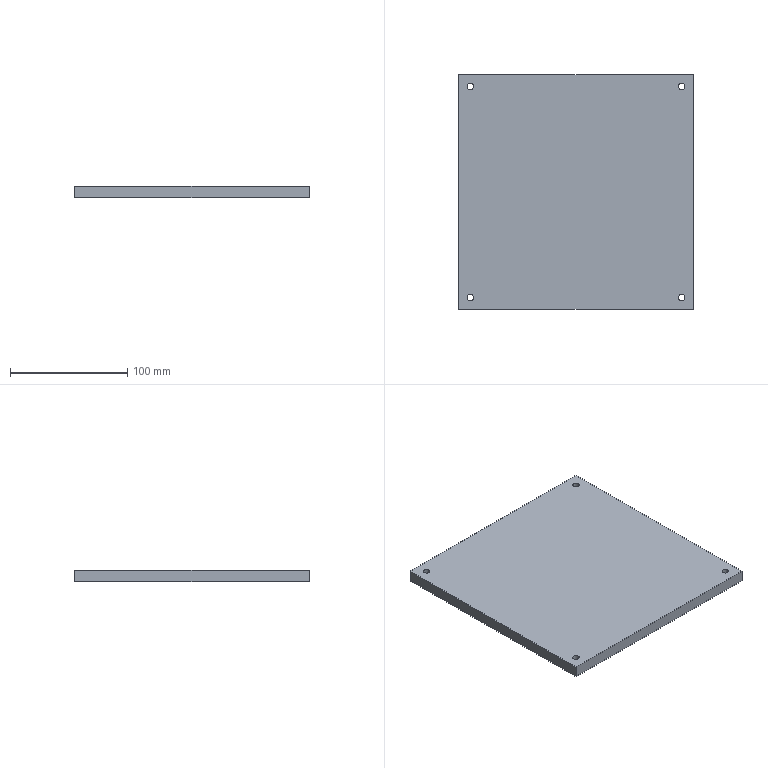Part | STEP file | B1-018 | 1 solid | 14 faces | box 200 x 200 x 10 mm | volume 399050 mm3 | cylinder 8 | plane 6 | commonest cylinder face diameters 5.5 x8
STEP:
#1=CARTESIAN_POINT('',(0.,0.,0.));
#2=DIRECTION('',(0.,0.,1.));
#3=DIRECTION('',(1.,0.,0.));
#4=AXIS2_PLACEMENT_3D('',#1,#2,#3);
#5=CARTESIAN_POINT('',(-87.25,90.,-5.));
#6=VERTEX_POINT('',#5);
#7=CARTESIAN_POINT('',(-87.25,90.,5.));
#8=VERTEX_POINT('',#7);
#9=CARTESIAN_POINT('',(-87.25,90.,-12.778));
#10=DIRECTION('',(0.,0.,1.));
#11=VECTOR('',#10,1.);
#12=LINE('',#9,#11);
#13=CARTESIAN_POINT('',(-90.,90.,-12.778));
#14=DIRECTION('',(0.,0.,1.));
#15=DIRECTION('',(1.,0.,0.));
#16=AXIS2_PLACEMENT_3D('',#13,#14,#15);
#17=CYLINDRICAL_SURFACE('',#16,2.75);
#18=CARTESIAN_POINT('',(6.283,0.));
#19=DIRECTION('',(0.,1.));
#20=VECTOR('',#19,1.);
#21=LINE('',#18,#20);
#22=(GEOMETRIC_REPRESENTATION_CONTEXT(2)PARAMETRIC_REPRESENTATION_CONTEXT()REPRESENTATION_CONTEXT('',''));
#23=DEFINITIONAL_REPRESENTATION('',(#21),#22);
#24=PCURVE('',#17,#23);
#25=CARTESIAN_POINT('',(-90.,90.,-12.778));
#26=DIRECTION('',(0.,0.,1.));
#27=DIRECTION('',(1.,0.,0.));
#28=AXIS2_PLACEMENT_3D('',#25,#26,#27);
#29=CYLINDRICAL_SURFACE('',#28,2.75);
#30=CARTESIAN_POINT('',(0.,0.));
#31=DIRECTION('',(0.,1.));
#32=VECTOR('',#31,1.);
#33=LINE('',#30,#32);
#34=(GEOMETRIC_REPRESENTATION_CONTEXT(2)PARAMETRIC_REPRESENTATION_CONTEXT()REPRESENTATION_CONTEXT('',''));
#35=DEFINITIONAL_REPRESENTATION('',(#33),#34);
#36=PCURVE('',#29,#35);
#37=SURFACE_CURVE('',#12,(#24,#36),.PCURVE_S1.);
#38=EDGE_CURVE('',#6,#8,#37,.T.);
#39=ORIENTED_EDGE('',*,*,#38,.T.);
#40=CARTESIAN_POINT('',(-92.75,90.,5.));
#41=VERTEX_POINT('',#40);
#42=CARTESIAN_POINT('',(-90.,90.,5.));
#43=DIRECTION('',(0.,0.,1.));
#44=DIRECTION('',(1.,0.,0.));
#45=AXIS2_PLACEMENT_3D('',#42,#43,#44);
#46=CIRCLE('',#45,2.75);
#47=CARTESIAN_POINT('',(0.,17.778));
#48=DIRECTION('',(1.,0.));
#49=VECTOR('',#48,1.);
#50=LINE('',#47,#49);
#51=(GEOMETRIC_REPRESENTATION_CONTEXT(2)PARAMETRIC_REPRESENTATION_CONTEXT()REPRESENTATION_CONTEXT('',''));
#52=DEFINITIONAL_REPRESENTATION('',(#50),#51);
#53=PCURVE('',#17,#52);
#54=CARTESIAN_POINT('',(0.,0.,5.));
#55=DIRECTION('',(0.,0.,1.));
#56=DIRECTION('',(1.,0.,0.));
#57=AXIS2_PLACEMENT_3D('',#54,#55,#56);
#58=PLANE('',#57);
#59=CARTESIAN_POINT('',(-90.,90.));
#60=DIRECTION('',(1.,0.));
#61=AXIS2_PLACEMENT_2D('',#59,#60);
#62=CIRCLE('',#61,2.75);
#63=(GEOMETRIC_REPRESENTATION_CONTEXT(2)PARAMETRIC_REPRESENTATION_CONTEXT()REPRESENTATION_CONTEXT('',''));
#64=DEFINITIONAL_REPRESENTATION('',(#62),#63);
#65=PCURVE('',#58,#64);
#66=SURFACE_CURVE('',#46,(#53,#65),.PCURVE_S1.);
#67=EDGE_CURVE('',#41,#8,#66,.T.);
#68=ORIENTED_EDGE('',*,*,#67,.F.);
#69=CARTESIAN_POINT('',(-92.75,90.,-5.));
#70=VERTEX_POINT('',#69);
#71=CARTESIAN_POINT('',(-92.75,90.,-12.778));
#72=DIRECTION('',(0.,0.,1.));
#73=VECTOR('',#72,1.);
#74=LINE('',#71,#73);
#75=CARTESIAN_POINT('',(3.142,0.));
#76=DIRECTION('',(0.,1.));
#77=VECTOR('',#76,1.);
#78=LINE('',#75,#77);
#79=(GEOMETRIC_REPRESENTATION_CONTEXT(2)PARAMETRIC_REPRESENTATION_CONTEXT()REPRESENTATION_CONTEXT('',''));
#80=DEFINITIONAL_REPRESENTATION('',(#78),#79);
#81=PCURVE('',#17,#80);
#82=CARTESIAN_POINT('',(3.142,0.));
#83=DIRECTION('',(0.,1.));
#84=VECTOR('',#83,1.);
#85=LINE('',#82,#84);
#86=(GEOMETRIC_REPRESENTATION_CONTEXT(2)PARAMETRIC_REPRESENTATION_CONTEXT()REPRESENTATION_CONTEXT('',''));
#87=DEFINITIONAL_REPRESENTATION('',(#85),#86);
#88=PCURVE('',#29,#87);
#89=SURFACE_CURVE('',#74,(#81,#88),.PCURVE_S1.);
#90=EDGE_CURVE('',#70,#41,#89,.T.);
#91=ORIENTED_EDGE('',*,*,#90,.F.);
#92=CARTESIAN_POINT('',(-90.,90.,-5.));
#93=DIRECTION('',(0.,0.,-1.));
#94=DIRECTION('',(1.,0.,0.));
#95=AXIS2_PLACEMENT_3D('',#92,#93,#94);
#96=CIRCLE('',#95,2.75);
#97=CARTESIAN_POINT('',(6.283,7.778));
#98=DIRECTION('',(-1.,0.));
#99=VECTOR('',#98,1.);
#100=LINE('',#97,#99);
#101=(GEOMETRIC_REPRESENTATION_CONTEXT(2)PARAMETRIC_REPRESENTATION_CONTEXT()REPRESENTATION_CONTEXT('',''));
#102=DEFINITIONAL_REPRESENTATION('',(#100),#101);
#103=PCURVE('',#17,#102);
#104=CARTESIAN_POINT('',(0.,0.,-5.));
#105=DIRECTION('',(0.,0.,1.));
#106=DIRECTION('',(1.,0.,0.));
#107=AXIS2_PLACEMENT_3D('',#104,#105,#106);
#108=PLANE('',#107);
#109=CARTESIAN_POINT('',(-87.25,90.));
#110=CARTESIAN_POINT('',(-87.25,85.237));
#111=CARTESIAN_POINT('',(-91.375,87.618));
#112=CARTESIAN_POINT('',(-95.5,90.));
#113=CARTESIAN_POINT('',(-91.375,92.382));
#114=CARTESIAN_POINT('',(-87.25,94.763));
#115=CARTESIAN_POINT('',(-87.25,90.));
#116=(BOUNDED_CURVE()B_SPLINE_CURVE(2,(#109,#110,#111,#112,#113,#114,#115),.UNSPECIFIED.,.T.,.F.)B_SPLINE_CURVE_WITH_KNOTS((1,2,2,2,2,1),(-2.094,0.,2.094,4.189,6.283,8.378),.UNSPECIFIED.)CURVE()GEOMETRIC_REPRESENTATION_ITEM()RATIONAL_B_SPLINE_CURVE((1.,0.5,1.,0.5,1.,0.5,1.))REPRESENTATION_ITEM(''));
#117=(GEOMETRIC_REPRESENTATION_CONTEXT(2)PARAMETRIC_REPRESENTATION_CONTEXT()REPRESENTATION_CONTEXT('',''));
#118=DEFINITIONAL_REPRESENTATION('',(#116),#117);
#119=PCURVE('',#108,#118);
#120=SURFACE_CURVE('',#96,(#103,#119),.PCURVE_S1.);
#121=EDGE_CURVE('',#6,#70,#120,.T.);
#122=ORIENTED_EDGE('',*,*,#121,.F.);
#123=EDGE_LOOP('',(#39,#68,#91,#122));
#124=FACE_BOUND('',#123,.F.);
#125=ADVANCED_FACE('',(#124),#17,.F.);
#126=CARTESIAN_POINT('',(-87.25,-90.,-5.));
#127=VERTEX_POINT('',#126);
#128=CARTESIAN_POINT('',(-87.25,-90.,5.));
#129=VERTEX_POINT('',#128);
#130=CARTESIAN_POINT('',(-87.25,-90.,-12.778));
#131=DIRECTION('',(0.,0.,1.));
#132=VECTOR('',#131,1.);
#133=LINE('',#130,#132);
#134=CARTESIAN_POINT('',(-90.,-90.,-12.778));
#135=DIRECTION('',(0.,0.,1.));
#136=DIRECTION('',(1.,0.,0.));
#137=AXIS2_PLACEMENT_3D('',#134,#135,#136);
#138=CYLINDRICAL_SURFACE('',#137,2.75);
#139=CARTESIAN_POINT('',(6.283,0.));
#140=DIRECTION('',(0.,1.));
#141=VECTOR('',#140,1.);
#142=LINE('',#139,#141);
#143=(GEOMETRIC_REPRESENTATION_CONTEXT(2)PARAMETRIC_REPRESENTATION_CONTEXT()REPRESENTATION_CONTEXT('',''));
#144=DEFINITIONAL_REPRESENTATION('',(#142),#143);
#145=PCURVE('',#138,#144);
#146=CARTESIAN_POINT('',(-90.,-90.,-12.778));
#147=DIRECTION('',(0.,0.,1.));
#148=DIRECTION('',(1.,0.,0.));
#149=AXIS2_PLACEMENT_3D('',#146,#147,#148);
#150=CYLINDRICAL_SURFACE('',#149,2.75);
#151=CARTESIAN_POINT('',(0.,0.));
#152=DIRECTION('',(0.,1.));
#153=VECTOR('',#152,1.);
#154=LINE('',#151,#153);
#155=(GEOMETRIC_REPRESENTATION_CONTEXT(2)PARAMETRIC_REPRESENTATION_CONTEXT()REPRESENTATION_CONTEXT('',''));
#156=DEFINITIONAL_REPRESENTATION('',(#154),#155);
#157=PCURVE('',#150,#156);
#158=SURFACE_CURVE('',#133,(#145,#157),.PCURVE_S1.);
#159=EDGE_CURVE('',#127,#129,#158,.T.);
#160=ORIENTED_EDGE('',*,*,#159,.T.);
#161=CARTESIAN_POINT('',(-92.75,-90.,5.));
#162=VERTEX_POINT('',#161);
#163=CARTESIAN_POINT('',(-90.,-90.,5.));
#164=DIRECTION('',(0.,0.,1.));
#165=DIRECTION('',(1.,0.,0.));
#166=AXIS2_PLACEMENT_3D('',#163,#164,#165);
#167=CIRCLE('',#166,2.75);
#168=CARTESIAN_POINT('',(0.,17.778));
#169=DIRECTION('',(1.,0.));
#170=VECTOR('',#169,1.);
#171=LINE('',#168,#170);
#172=(GEOMETRIC_REPRESENTATION_CONTEXT(2)PARAMETRIC_REPRESENTATION_CONTEXT()REPRESENTATION_CONTEXT('',''));
#173=DEFINITIONAL_REPRESENTATION('',(#171),#172);
#174=PCURVE('',#138,#173);
#175=CARTESIAN_POINT('',(-90.,-90.));
#176=DIRECTION('',(1.,0.));
#177=AXIS2_PLACEMENT_2D('',#175,#176);
#178=CIRCLE('',#177,2.75);
#179=(GEOMETRIC_REPRESENTATION_CONTEXT(2)PARAMETRIC_REPRESENTATION_CONTEXT()REPRESENTATION_CONTEXT('',''));
#180=DEFINITIONAL_REPRESENTATION('',(#178),#179);
#181=PCURVE('',#58,#180);
#182=SURFACE_CURVE('',#167,(#174,#181),.PCURVE_S1.);
#183=EDGE_CURVE('',#162,#129,#182,.T.);
#184=ORIENTED_EDGE('',*,*,#183,.F.);
#185=CARTESIAN_POINT('',(-92.75,-90.,-5.));
#186=VERTEX_POINT('',#185);
#187=CARTESIAN_POINT('',(-92.75,-90.,-12.778));
#188=DIRECTION('',(0.,0.,1.));
#189=VECTOR('',#188,1.);
#190=LINE('',#187,#189);
#191=CARTESIAN_POINT('',(3.142,0.));
#192=DIRECTION('',(0.,1.));
#193=VECTOR('',#192,1.);
#194=LINE('',#191,#193);
#195=(GEOMETRIC_REPRESENTATION_CONTEXT(2)PARAMETRIC_REPRESENTATION_CONTEXT()REPRESENTATION_CONTEXT('',''));
#196=DEFINITIONAL_REPRESENTATION('',(#194),#195);
#197=PCURVE('',#138,#196);
#198=CARTESIAN_POINT('',(3.142,0.));
#199=DIRECTION('',(0.,1.));
#200=VECTOR('',#199,1.);
#201=LINE('',#198,#200);
#202=(GEOMETRIC_REPRESENTATION_CONTEXT(2)PARAMETRIC_REPRESENTATION_CONTEXT()REPRESENTATION_CONTEXT('',''));
#203=DEFINITIONAL_REPRESENTATION('',(#201),#202);
#204=PCURVE('',#150,#203);
#205=SURFACE_CURVE('',#190,(#197,#204),.PCURVE_S1.);
#206=EDGE_CURVE('',#186,#162,#205,.T.);
#207=ORIENTED_EDGE('',*,*,#206,.F.);
#208=CARTESIAN_POINT('',(-90.,-90.,-5.));
#209=DIRECTION('',(0.,0.,-1.));
#210=DIRECTION('',(1.,0.,0.));
#211=AXIS2_PLACEMENT_3D('',#208,#209,#210);
#212=CIRCLE('',#211,2.75);
#213=CARTESIAN_POINT('',(6.283,7.778));
#214=DIRECTION('',(-1.,0.));
#215=VECTOR('',#214,1.);
#216=LINE('',#213,#215);
#217=(GEOMETRIC_REPRESENTATION_CONTEXT(2)PARAMETRIC_REPRESENTATION_CONTEXT()REPRESENTATION_CONTEXT('',''));
#218=DEFINITIONAL_REPRESENTATION('',(#216),#217);
#219=PCURVE('',#138,#218);
#220=CARTESIAN_POINT('',(-87.25,-90.));
#221=CARTESIAN_POINT('',(-87.25,-94.763));
#222=CARTESIAN_POINT('',(-91.375,-92.382));
#223=CARTESIAN_POINT('',(-95.5,-90.));
#224=CARTESIAN_POINT('',(-91.375,-87.618));
#225=CARTESIAN_POINT('',(-87.25,-85.237));
#226=CARTESIAN_POINT('',(-87.25,-90.));
#227=(BOUNDED_CURVE()B_SPLINE_CURVE(2,(#220,#221,#222,#223,#224,#225,#226),.UNSPECIFIED.,.T.,.F.)B_SPLINE_CURVE_WITH_KNOTS((1,2,2,2,2,1),(-2.094,0.,2.094,4.189,6.283,8.378),.UNSPECIFIED.)CURVE()GEOMETRIC_REPRESENTATION_ITEM()RATIONAL_B_SPLINE_CURVE((1.,0.5,1.,0.5,1.,0.5,1.))REPRESENTATION_ITEM(''));
#228=(GEOMETRIC_REPRESENTATION_CONTEXT(2)PARAMETRIC_REPRESENTATION_CONTEXT()REPRESENTATION_CONTEXT('',''));
#229=DEFINITIONAL_REPRESENTATION('',(#227),#228);
#230=PCURVE('',#108,#229);
#231=SURFACE_CURVE('',#212,(#219,#230),.PCURVE_S1.);
#232=EDGE_CURVE('',#127,#186,#231,.T.);
#233=ORIENTED_EDGE('',*,*,#232,.F.);
#234=EDGE_LOOP('',(#160,#184,#207,#233));
#235=FACE_BOUND('',#234,.F.);
#236=ADVANCED_FACE('',(#235),#138,.F.);
#237=CARTESIAN_POINT('',(92.75,-90.,-5.));
#238=VERTEX_POINT('',#237);
#239=CARTESIAN_POINT('',(92.75,-90.,5.));
#240=VERTEX_POINT('',#239);
#241=CARTESIAN_POINT('',(92.75,-90.,-12.778));
#242=DIRECTION('',(0.,0.,1.));
#243=VECTOR('',#242,1.);
#244=LINE('',#241,#243);
#245=CARTESIAN_POINT('',(90.,-90.,-12.778));
#246=DIRECTION('',(0.,0.,1.));
#247=DIRECTION('',(1.,0.,0.));
#248=AXIS2_PLACEMENT_3D('',#245,#246,#247);
#249=CYLINDRICAL_SURFACE('',#248,2.75);
#250=CARTESIAN_POINT('',(6.283,0.));
#251=DIRECTION('',(0.,1.));
#252=VECTOR('',#251,1.);
#253=LINE('',#250,#252);
#254=(GEOMETRIC_REPRESENTATION_CONTEXT(2)PARAMETRIC_REPRESENTATION_CONTEXT()REPRESENTATION_CONTEXT('',''));
#255=DEFINITIONAL_REPRESENTATION('',(#253),#254);
#256=PCURVE('',#249,#255);
#257=CARTESIAN_POINT('',(90.,-90.,-12.778));
#258=DIRECTION('',(0.,0.,1.));
#259=DIRECTION('',(1.,0.,0.));
#260=AXIS2_PLACEMENT_3D('',#257,#258,#259);
#261=CYLINDRICAL_SURFACE('',#260,2.75);
#262=CARTESIAN_POINT('',(0.,0.));
#263=DIRECTION('',(0.,1.));
#264=VECTOR('',#263,1.);
#265=LINE('',#262,#264);
#266=(GEOMETRIC_REPRESENTATION_CONTEXT(2)PARAMETRIC_REPRESENTATION_CONTEXT()REPRESENTATION_CONTEXT('',''));
#267=DEFINITIONAL_REPRESENTATION('',(#265),#266);
#268=PCURVE('',#261,#267);
#269=SURFACE_CURVE('',#244,(#256,#268),.PCURVE_S1.);
#270=EDGE_CURVE('',#238,#240,#269,.T.);
#271=ORIENTED_EDGE('',*,*,#270,.T.);
#272=CARTESIAN_POINT('',(87.25,-90.,5.));
#273=VERTEX_POINT('',#272);
#274=CARTESIAN_POINT('',(90.,-90.,5.));
#275=DIRECTION('',(0.,0.,1.));
#276=DIRECTION('',(1.,0.,0.));
#277=AXIS2_PLACEMENT_3D('',#274,#275,#276);
#278=CIRCLE('',#277,2.75);
#279=CARTESIAN_POINT('',(0.,17.778));
#280=DIRECTION('',(1.,0.));
#281=VECTOR('',#280,1.);
#282=LINE('',#279,#281);
#283=(GEOMETRIC_REPRESENTATION_CONTEXT(2)PARAMETRIC_REPRESENTATION_CONTEXT()REPRESENTATION_CONTEXT('',''));
#284=DEFINITIONAL_REPRESENTATION('',(#282),#283);
#285=PCURVE('',#249,#284);
#286=CARTESIAN_POINT('',(90.,-90.));
#287=DIRECTION('',(1.,0.));
#288=AXIS2_PLACEMENT_2D('',#286,#287);
#289=CIRCLE('',#288,2.75);
#290=(GEOMETRIC_REPRESENTATION_CONTEXT(2)PARAMETRIC_REPRESENTATION_CONTEXT()REPRESENTATION_CONTEXT('',''));
#291=DEFINITIONAL_REPRESENTATION('',(#289),#290);
#292=PCURVE('',#58,#291);
#293=SURFACE_CURVE('',#278,(#285,#292),.PCURVE_S1.);
#294=EDGE_CURVE('',#273,#240,#293,.T.);
#295=ORIENTED_EDGE('',*,*,#294,.F.);
#296=CARTESIAN_POINT('',(87.25,-90.,-5.));
#297=VERTEX_POINT('',#296);
#298=CARTESIAN_POINT('',(87.25,-90.,-12.778));
#299=DIRECTION('',(0.,0.,1.));
#300=VECTOR('',#299,1.);
#301=LINE('',#298,#300);
#302=CARTESIAN_POINT('',(3.142,0.));
#303=DIRECTION('',(0.,1.));
#304=VECTOR('',#303,1.);
#305=LINE('',#302,#304);
#306=(GEOMETRIC_REPRESENTATION_CONTEXT(2)PARAMETRIC_REPRESENTATION_CONTEXT()REPRESENTATION_CONTEXT('',''));
#307=DEFINITIONAL_REPRESENTATION('',(#305),#306);
#308=PCURVE('',#249,#307);
#309=CARTESIAN_POINT('',(3.142,0.));
#310=DIRECTION('',(0.,1.));
#311=VECTOR('',#310,1.);
#312=LINE('',#309,#311);
#313=(GEOMETRIC_REPRESENTATION_CONTEXT(2)PARAMETRIC_REPRESENTATION_CONTEXT()REPRESENTATION_CONTEXT('',''));
#314=DEFINITIONAL_REPRESENTATION('',(#312),#313);
#315=PCURVE('',#261,#314);
#316=SURFACE_CURVE('',#301,(#308,#315),.PCURVE_S1.);
#317=EDGE_CURVE('',#297,#273,#316,.T.);
#318=ORIENTED_EDGE('',*,*,#317,.F.);
#319=CARTESIAN_POINT('',(90.,-90.,-5.));
#320=DIRECTION('',(0.,0.,-1.));
#321=DIRECTION('',(1.,0.,0.));
#322=AXIS2_PLACEMENT_3D('',#319,#320,#321);
#323=CIRCLE('',#322,2.75);
#324=CARTESIAN_POINT('',(6.283,7.778));
#325=DIRECTION('',(-1.,0.));
#326=VECTOR('',#325,1.);
#327=LINE('',#324,#326);
#328=(GEOMETRIC_REPRESENTATION_CONTEXT(2)PARAMETRIC_REPRESENTATION_CONTEXT()REPRESENTATION_CONTEXT('',''));
#329=DEFINITIONAL_REPRESENTATION('',(#327),#328);
#330=PCURVE('',#249,#329);
#331=CARTESIAN_POINT('',(92.75,-90.));
#332=CARTESIAN_POINT('',(92.75,-94.763));
#333=CARTESIAN_POINT('',(88.625,-92.382));
#334=CARTESIAN_POINT('',(84.5,-90.));
#335=CARTESIAN_POINT('',(88.625,-87.618));
#336=CARTESIAN_POINT('',(92.75,-85.237));
#337=CARTESIAN_POINT('',(92.75,-90.));
#338=(BOUNDED_CURVE()B_SPLINE_CURVE(2,(#331,#332,#333,#334,#335,#336,#337),.UNSPECIFIED.,.T.,.F.)B_SPLINE_CURVE_WITH_KNOTS((1,2,2,2,2,1),(-2.094,0.,2.094,4.189,6.283,8.378),.UNSPECIFIED.)CURVE()GEOMETRIC_REPRESENTATION_ITEM()RATIONAL_B_SPLINE_CURVE((1.,0.5,1.,0.5,1.,0.5,1.))REPRESENTATION_ITEM(''));
#339=(GEOMETRIC_REPRESENTATION_CONTEXT(2)PARAMETRIC_REPRESENTATION_CONTEXT()REPRESENTATION_CONTEXT('',''));
#340=DEFINITIONAL_REPRESENTATION('',(#338),#339);
#341=PCURVE('',#108,#340);
#342=SURFACE_CURVE('',#323,(#330,#341),.PCURVE_S1.);
#343=EDGE_CURVE('',#238,#297,#342,.T.);
#344=ORIENTED_EDGE('',*,*,#343,.F.);
#345=EDGE_LOOP('',(#271,#295,#318,#344));
#346=FACE_BOUND('',#345,.F.);
#347=ADVANCED_FACE('',(#346),#249,.F.);
#348=CARTESIAN_POINT('',(92.75,90.,-5.));
#349=VERTEX_POINT('',#348);
#350=CARTESIAN_POINT('',(92.75,90.,5.));
#351=VERTEX_POINT('',#350);
#352=CARTESIAN_POINT('',(92.75,90.,-12.778));
#353=DIRECTION('',(0.,0.,1.));
#354=VECTOR('',#353,1.);
#355=LINE('',#352,#354);
#356=CARTESIAN_POINT('',(90.,90.,-12.778));
#357=DIRECTION('',(0.,0.,1.));
#358=DIRECTION('',(1.,0.,0.));
#359=AXIS2_PLACEMENT_3D('',#356,#357,#358);
#360=CYLINDRICAL_SURFACE('',#359,2.75);
#361=CARTESIAN_POINT('',(6.283,0.));
#362=DIRECTION('',(0.,1.));
#363=VECTOR('',#362,1.);
#364=LINE('',#361,#363);
#365=(GEOMETRIC_REPRESENTATION_CONTEXT(2)PARAMETRIC_REPRESENTATION_CONTEXT()REPRESENTATION_CONTEXT('',''));
#366=DEFINITIONAL_REPRESENTATION('',(#364),#365);
#367=PCURVE('',#360,#366);
#368=CARTESIAN_POINT('',(90.,90.,-12.778));
#369=DIRECTION('',(0.,0.,1.));
#370=DIRECTION('',(1.,0.,0.));
#371=AXIS2_PLACEMENT_3D('',#368,#369,#370);
#372=CYLINDRICAL_SURFACE('',#371,2.75);
#373=CARTESIAN_POINT('',(0.,0.));
#374=DIRECTION('',(0.,1.));
#375=VECTOR('',#374,1.);
#376=LINE('',#373,#375);
#377=(GEOMETRIC_REPRESENTATION_CONTEXT(2)PARAMETRIC_REPRESENTATION_CONTEXT()REPRESENTATION_CONTEXT('',''));
#378=DEFINITIONAL_REPRESENTATION('',(#376),#377);
#379=PCURVE('',#372,#378);
#380=SURFACE_CURVE('',#355,(#367,#379),.PCURVE_S1.);
#381=EDGE_CURVE('',#349,#351,#380,.T.);
#382=ORIENTED_EDGE('',*,*,#381,.T.);
#383=CARTESIAN_POINT('',(87.25,90.,5.));
#384=VERTEX_POINT('',#383);
#385=CARTESIAN_POINT('',(90.,90.,5.));
#386=DIRECTION('',(0.,0.,1.));
#387=DIRECTION('',(1.,0.,0.));
#388=AXIS2_PLACEMENT_3D('',#385,#386,#387);
#389=CIRCLE('',#388,2.75);
#390=CARTESIAN_POINT('',(0.,17.778));
#391=DIRECTION('',(1.,0.));
#392=VECTOR('',#391,1.);
#393=LINE('',#390,#392);
#394=(GEOMETRIC_REPRESENTATION_CONTEXT(2)PARAMETRIC_REPRESENTATION_CONTEXT()REPRESENTATION_CONTEXT('',''));
#395=DEFINITIONAL_REPRESENTATION('',(#393),#394);
#396=PCURVE('',#360,#395);
#397=CARTESIAN_POINT('',(90.,90.));
#398=DIRECTION('',(1.,0.));
#399=AXIS2_PLACEMENT_2D('',#397,#398);
#400=CIRCLE('',#399,2.75);
#401=(GEOMETRIC_REPRESENTATION_CONTEXT(2)PARAMETRIC_REPRESENTATION_CONTEXT()REPRESENTATION_CONTEXT('',''));
#402=DEFINITIONAL_REPRESENTATION('',(#400),#401);
#403=PCURVE('',#58,#402);
#404=SURFACE_CURVE('',#389,(#396,#403),.PCURVE_S1.);
#405=EDGE_CURVE('',#384,#351,#404,.T.);
#406=ORIENTED_EDGE('',*,*,#405,.F.);
#407=CARTESIAN_POINT('',(87.25,90.,-5.));
#408=VERTEX_POINT('',#407);
#409=CARTESIAN_POINT('',(87.25,90.,-12.778));
#410=DIRECTION('',(0.,0.,1.));
#411=VECTOR('',#410,1.);
#412=LINE('',#409,#411);
#413=CARTESIAN_POINT('',(3.142,0.));
#414=DIRECTION('',(0.,1.));
#415=VECTOR('',#414,1.);
#416=LINE('',#413,#415);
#417=(GEOMETRIC_REPRESENTATION_CONTEXT(2)PARAMETRIC_REPRESENTATION_CONTEXT()REPRESENTATION_CONTEXT('',''));
#418=DEFINITIONAL_REPRESENTATION('',(#416),#417);
#419=PCURVE('',#360,#418);
#420=CARTESIAN_POINT('',(3.142,0.));
#421=DIRECTION('',(0.,1.));
#422=VECTOR('',#421,1.);
#423=LINE('',#420,#422);
#424=(GEOMETRIC_REPRESENTATION_CONTEXT(2)PARAMETRIC_REPRESENTATION_CONTEXT()REPRESENTATION_CONTEXT('',''));
#425=DEFINITIONAL_REPRESENTATION('',(#423),#424);
#426=PCURVE('',#372,#425);
#427=SURFACE_CURVE('',#412,(#419,#426),.PCURVE_S1.);
#428=EDGE_CURVE('',#408,#384,#427,.T.);
#429=ORIENTED_EDGE('',*,*,#428,.F.);
#430=CARTESIAN_POINT('',(90.,90.,-5.));
#431=DIRECTION('',(0.,0.,-1.));
#432=DIRECTION('',(1.,0.,0.));
#433=AXIS2_PLACEMENT_3D('',#430,#431,#432);
#434=CIRCLE('',#433,2.75);
#435=CARTESIAN_POINT('',(6.283,7.778));
#436=DIRECTION('',(-1.,0.));
#437=VECTOR('',#436,1.);
#438=LINE('',#435,#437);
#439=(GEOMETRIC_REPRESENTATION_CONTEXT(2)PARAMETRIC_REPRESENTATION_CONTEXT()REPRESENTATION_CONTEXT('',''));
#440=DEFINITIONAL_REPRESENTATION('',(#438),#439);
#441=PCURVE('',#360,#440);
#442=CARTESIAN_POINT('',(92.75,90.));
#443=CARTESIAN_POINT('',(92.75,85.237));
#444=CARTESIAN_POINT('',(88.625,87.618));
#445=CARTESIAN_POINT('',(84.5,90.));
#446=CARTESIAN_POINT('',(88.625,92.382));
#447=CARTESIAN_POINT('',(92.75,94.763));
#448=CARTESIAN_POINT('',(92.75,90.));
#449=(BOUNDED_CURVE()B_SPLINE_CURVE(2,(#442,#443,#444,#445,#446,#447,#448),.UNSPECIFIED.,.T.,.F.)B_SPLINE_CURVE_WITH_KNOTS((1,2,2,2,2,1),(-2.094,0.,2.094,4.189,6.283,8.378),.UNSPECIFIED.)CURVE()GEOMETRIC_REPRESENTATION_ITEM()RATIONAL_B_SPLINE_CURVE((1.,0.5,1.,0.5,1.,0.5,1.))REPRESENTATION_ITEM(''));
#450=(GEOMETRIC_REPRESENTATION_CONTEXT(2)PARAMETRIC_REPRESENTATION_CONTEXT()REPRESENTATION_CONTEXT('',''));
#451=DEFINITIONAL_REPRESENTATION('',(#449),#450);
#452=PCURVE('',#108,#451);
#453=SURFACE_CURVE('',#434,(#441,#452),.PCURVE_S1.);
#454=EDGE_CURVE('',#349,#408,#453,.T.);
#455=ORIENTED_EDGE('',*,*,#454,.F.);
#456=EDGE_LOOP('',(#382,#406,#429,#455));
#457=FACE_BOUND('',#456,.F.);
#458=ADVANCED_FACE('',(#457),#360,.F.);
#459=CARTESIAN_POINT('',(100.,-100.,-5.));
#460=VERTEX_POINT('',#459);
#461=CARTESIAN_POINT('',(100.,100.,-5.));
#462=VERTEX_POINT('',#461);
#463=CARTESIAN_POINT('',(100.,100.,-5.));
#464=DIRECTION('',(0.,1.,0.));
#465=VECTOR('',#464,1.);
#466=LINE('',#463,#465);
#467=CARTESIAN_POINT('',(100.,100.,5.));
#468=DIRECTION('',(-1.,0.,0.));
#469=DIRECTION('',(0.,0.,1.));
#470=AXIS2_PLACEMENT_3D('',#467,#468,#469);
#471=PLANE('',#470);
#472=CARTESIAN_POINT('',(-10.,0.));
#473=DIRECTION('',(0.,1.));
#474=VECTOR('',#473,1.);
#475=LINE('',#472,#474);
#476=(GEOMETRIC_REPRESENTATION_CONTEXT(2)PARAMETRIC_REPRESENTATION_CONTEXT()REPRESENTATION_CONTEXT('',''));
#477=DEFINITIONAL_REPRESENTATION('',(#475),#476);
#478=PCURVE('',#471,#477);
#479=CARTESIAN_POINT('',(100.,100.));
#480=DIRECTION('',(0.,1.));
#481=VECTOR('',#480,1.);
#482=LINE('',#479,#481);
#483=(GEOMETRIC_REPRESENTATION_CONTEXT(2)PARAMETRIC_REPRESENTATION_CONTEXT()REPRESENTATION_CONTEXT('',''));
#484=DEFINITIONAL_REPRESENTATION('',(#482),#483);
#485=PCURVE('',#108,#484);
#486=SURFACE_CURVE('',#466,(#478,#485),.PCURVE_S1.);
#487=EDGE_CURVE('',#460,#462,#486,.T.);
#488=ORIENTED_EDGE('',*,*,#487,.T.);
#489=CARTESIAN_POINT('',(100.,100.,5.));
#490=VERTEX_POINT('',#489);
#491=CARTESIAN_POINT('',(100.,100.,5.));
#492=DIRECTION('',(0.,0.,-1.));
#493=VECTOR('',#492,1.);
#494=LINE('',#491,#493);
#495=CARTESIAN_POINT('',(0.,0.));
#496=DIRECTION('',(-1.,0.));
#497=VECTOR('',#496,1.);
#498=LINE('',#495,#497);
#499=(GEOMETRIC_REPRESENTATION_CONTEXT(2)PARAMETRIC_REPRESENTATION_CONTEXT()REPRESENTATION_CONTEXT('',''));
#500=DEFINITIONAL_REPRESENTATION('',(#498),#499);
#501=PCURVE('',#471,#500);
#502=CARTESIAN_POINT('',(-100.,100.,5.));
#503=DIRECTION('',(0.,-1.,0.));
#504=DIRECTION('',(0.,0.,-1.));
#505=AXIS2_PLACEMENT_3D('',#502,#503,#504);
#506=PLANE('',#505);
#507=CARTESIAN_POINT('',(0.,200.));
#508=DIRECTION('',(1.,0.));
#509=VECTOR('',#508,1.);
#510=LINE('',#507,#509);
#511=(GEOMETRIC_REPRESENTATION_CONTEXT(2)PARAMETRIC_REPRESENTATION_CONTEXT()REPRESENTATION_CONTEXT('',''));
#512=DEFINITIONAL_REPRESENTATION('',(#510),#511);
#513=PCURVE('',#506,#512);
#514=SURFACE_CURVE('',#494,(#501,#513),.PCURVE_S1.);
#515=EDGE_CURVE('',#490,#462,#514,.T.);
#516=ORIENTED_EDGE('',*,*,#515,.F.);
#517=CARTESIAN_POINT('',(100.,-100.,5.));
#518=VERTEX_POINT('',#517);
#519=CARTESIAN_POINT('',(100.,100.,5.));
#520=DIRECTION('',(0.,1.,0.));
#521=VECTOR('',#520,1.);
#522=LINE('',#519,#521);
#523=CARTESIAN_POINT('',(0.,0.));
#524=DIRECTION('',(0.,1.));
#525=VECTOR('',#524,1.);
#526=LINE('',#523,#525);
#527=(GEOMETRIC_REPRESENTATION_CONTEXT(2)PARAMETRIC_REPRESENTATION_CONTEXT()REPRESENTATION_CONTEXT('',''));
#528=DEFINITIONAL_REPRESENTATION('',(#526),#527);
#529=PCURVE('',#471,#528);
#530=CARTESIAN_POINT('',(100.,100.));
#531=DIRECTION('',(0.,1.));
#532=VECTOR('',#531,1.);
#533=LINE('',#530,#532);
#534=(GEOMETRIC_REPRESENTATION_CONTEXT(2)PARAMETRIC_REPRESENTATION_CONTEXT()REPRESENTATION_CONTEXT('',''));
#535=DEFINITIONAL_REPRESENTATION('',(#533),#534);
#536=PCURVE('',#58,#535);
#537=SURFACE_CURVE('',#522,(#529,#536),.PCURVE_S1.);
#538=EDGE_CURVE('',#518,#490,#537,.T.);
#539=ORIENTED_EDGE('',*,*,#538,.F.);
#540=CARTESIAN_POINT('',(100.,-100.,5.));
#541=DIRECTION('',(0.,0.,-1.));
#542=VECTOR('',#541,1.);
#543=LINE('',#540,#542);
#544=CARTESIAN_POINT('',(0.,-200.));
#545=DIRECTION('',(-1.,0.));
#546=VECTOR('',#545,1.);
#547=LINE('',#544,#546);
#548=(GEOMETRIC_REPRESENTATION_CONTEXT(2)PARAMETRIC_REPRESENTATION_CONTEXT()REPRESENTATION_CONTEXT('',''));
#549=DEFINITIONAL_REPRESENTATION('',(#547),#548);
#550=PCURVE('',#471,#549);
#551=CARTESIAN_POINT('',(-100.,-100.,5.));
#552=DIRECTION('',(0.,1.,0.));
#553=DIRECTION('',(0.,0.,1.));
#554=AXIS2_PLACEMENT_3D('',#551,#552,#553);
#555=PLANE('',#554);
#556=CARTESIAN_POINT('',(0.,200.));
#557=DIRECTION('',(-1.,0.));
#558=VECTOR('',#557,1.);
#559=LINE('',#556,#558);
#560=(GEOMETRIC_REPRESENTATION_CONTEXT(2)PARAMETRIC_REPRESENTATION_CONTEXT()REPRESENTATION_CONTEXT('',''));
#561=DEFINITIONAL_REPRESENTATION('',(#559),#560);
#562=PCURVE('',#555,#561);
#563=SURFACE_CURVE('',#543,(#550,#562),.PCURVE_S1.);
#564=EDGE_CURVE('',#518,#460,#563,.T.);
#565=ORIENTED_EDGE('',*,*,#564,.T.);
#566=EDGE_LOOP('',(#488,#516,#539,#565));
#567=FACE_BOUND('',#566,.T.);
#568=ADVANCED_FACE('',(#567),#471,.F.);
#569=CARTESIAN_POINT('',(-100.,100.,-5.));
#570=VERTEX_POINT('',#569);
#571=CARTESIAN_POINT('',(-100.,100.,-5.));
#572=DIRECTION('',(-1.,0.,0.));
#573=VECTOR('',#572,1.);
#574=LINE('',#571,#573);
#575=CARTESIAN_POINT('',(10.,0.));
#576=DIRECTION('',(0.,-1.));
#577=VECTOR('',#576,1.);
#578=LINE('',#575,#577);
#579=(GEOMETRIC_REPRESENTATION_CONTEXT(2)PARAMETRIC_REPRESENTATION_CONTEXT()REPRESENTATION_CONTEXT('',''));
#580=DEFINITIONAL_REPRESENTATION('',(#578),#579);
#581=PCURVE('',#506,#580);
#582=CARTESIAN_POINT('',(-100.,100.));
#583=DIRECTION('',(-1.,0.));
#584=VECTOR('',#583,1.);
#585=LINE('',#582,#584);
#586=(GEOMETRIC_REPRESENTATION_CONTEXT(2)PARAMETRIC_REPRESENTATION_CONTEXT()REPRESENTATION_CONTEXT('',''));
#587=DEFINITIONAL_REPRESENTATION('',(#585),#586);
#588=PCURVE('',#108,#587);
#589=SURFACE_CURVE('',#574,(#581,#588),.PCURVE_S1.);
#590=EDGE_CURVE('',#462,#570,#589,.T.);
#591=ORIENTED_EDGE('',*,*,#590,.T.);
#592=CARTESIAN_POINT('',(-100.,100.,5.));
#593=VERTEX_POINT('',#592);
#594=CARTESIAN_POINT('',(-100.,100.,5.));
#595=DIRECTION('',(0.,0.,-1.));
#596=VECTOR('',#595,1.);
#597=LINE('',#594,#596);
#598=CARTESIAN_POINT('',(0.,0.));
#599=DIRECTION('',(1.,0.));
#600=VECTOR('',#599,1.);
#601=LINE('',#598,#600);
#602=(GEOMETRIC_REPRESENTATION_CONTEXT(2)PARAMETRIC_REPRESENTATION_CONTEXT()REPRESENTATION_CONTEXT('',''));
#603=DEFINITIONAL_REPRESENTATION('',(#601),#602);
#604=PCURVE('',#506,#603);
#605=CARTESIAN_POINT('',(-100.,100.,5.));
#606=DIRECTION('',(1.,0.,0.));
#607=DIRECTION('',(0.,0.,-1.));
#608=AXIS2_PLACEMENT_3D('',#605,#606,#607);
#609=PLANE('',#608);
#610=CARTESIAN_POINT('',(0.,0.));
#611=DIRECTION('',(1.,0.));
#612=VECTOR('',#611,1.);
#613=LINE('',#610,#612);
#614=(GEOMETRIC_REPRESENTATION_CONTEXT(2)PARAMETRIC_REPRESENTATION_CONTEXT()REPRESENTATION_CONTEXT('',''));
#615=DEFINITIONAL_REPRESENTATION('',(#613),#614);
#616=PCURVE('',#609,#615);
#617=SURFACE_CURVE('',#597,(#604,#616),.PCURVE_S1.);
#618=EDGE_CURVE('',#593,#570,#617,.T.);
#619=ORIENTED_EDGE('',*,*,#618,.F.);
#620=CARTESIAN_POINT('',(-100.,100.,5.));
#621=DIRECTION('',(-1.,0.,0.));
#622=VECTOR('',#621,1.);
#623=LINE('',#620,#622);
#624=CARTESIAN_POINT('',(0.,0.));
#625=DIRECTION('',(0.,-1.));
#626=VECTOR('',#625,1.);
#627=LINE('',#624,#626);
#628=(GEOMETRIC_REPRESENTATION_CONTEXT(2)PARAMETRIC_REPRESENTATION_CONTEXT()REPRESENTATION_CONTEXT('',''));
#629=DEFINITIONAL_REPRESENTATION('',(#627),#628);
#630=PCURVE('',#506,#629);
#631=CARTESIAN_POINT('',(-100.,100.));
#632=DIRECTION('',(-1.,0.));
#633=VECTOR('',#632,1.);
#634=LINE('',#631,#633);
#635=(GEOMETRIC_REPRESENTATION_CONTEXT(2)PARAMETRIC_REPRESENTATION_CONTEXT()REPRESENTATION_CONTEXT('',''));
#636=DEFINITIONAL_REPRESENTATION('',(#634),#635);
#637=PCURVE('',#58,#636);
#638=SURFACE_CURVE('',#623,(#630,#637),.PCURVE_S1.);
#639=EDGE_CURVE('',#490,#593,#638,.T.);
#640=ORIENTED_EDGE('',*,*,#639,.F.);
#641=ORIENTED_EDGE('',*,*,#515,.T.);
#642=EDGE_LOOP('',(#591,#619,#640,#641));
#643=FACE_BOUND('',#642,.T.);
#644=ADVANCED_FACE('',(#643),#506,.F.);
#645=CARTESIAN_POINT('',(-100.,-100.,-5.));
#646=VERTEX_POINT('',#645);
#647=CARTESIAN_POINT('',(-100.,100.,-5.));
#648=DIRECTION('',(0.,-1.,0.));
#649=VECTOR('',#648,1.);
#650=LINE('',#647,#649);
#651=CARTESIAN_POINT('',(10.,0.));
#652=DIRECTION('',(0.,-1.));
#653=VECTOR('',#652,1.);
#654=LINE('',#651,#653);
#655=(GEOMETRIC_REPRESENTATION_CONTEXT(2)PARAMETRIC_REPRESENTATION_CONTEXT()REPRESENTATION_CONTEXT('',''));
#656=DEFINITIONAL_REPRESENTATION('',(#654),#655);
#657=PCURVE('',#609,#656);
#658=CARTESIAN_POINT('',(-100.,100.));
#659=DIRECTION('',(0.,-1.));
#660=VECTOR('',#659,1.);
#661=LINE('',#658,#660);
#662=(GEOMETRIC_REPRESENTATION_CONTEXT(2)PARAMETRIC_REPRESENTATION_CONTEXT()REPRESENTATION_CONTEXT('',''));
#663=DEFINITIONAL_REPRESENTATION('',(#661),#662);
#664=PCURVE('',#108,#663);
#665=SURFACE_CURVE('',#650,(#657,#664),.PCURVE_S1.);
#666=EDGE_CURVE('',#570,#646,#665,.T.);
#667=ORIENTED_EDGE('',*,*,#666,.T.);
#668=CARTESIAN_POINT('',(-100.,-100.,5.));
#669=VERTEX_POINT('',#668);
#670=CARTESIAN_POINT('',(-100.,-100.,5.));
#671=DIRECTION('',(0.,0.,-1.));
#672=VECTOR('',#671,1.);
#673=LINE('',#670,#672);
#674=CARTESIAN_POINT('',(0.,-200.));
#675=DIRECTION('',(1.,0.));
#676=VECTOR('',#675,1.);
#677=LINE('',#674,#676);
#678=(GEOMETRIC_REPRESENTATION_CONTEXT(2)PARAMETRIC_REPRESENTATION_CONTEXT()REPRESENTATION_CONTEXT('',''));
#679=DEFINITIONAL_REPRESENTATION('',(#677),#678);
#680=PCURVE('',#609,#679);
#681=CARTESIAN_POINT('',(0.,0.));
#682=DIRECTION('',(-1.,0.));
#683=VECTOR('',#682,1.);
#684=LINE('',#681,#683);
#685=(GEOMETRIC_REPRESENTATION_CONTEXT(2)PARAMETRIC_REPRESENTATION_CONTEXT()REPRESENTATION_CONTEXT('',''));
#686=DEFINITIONAL_REPRESENTATION('',(#684),#685);
#687=PCURVE('',#555,#686);
#688=SURFACE_CURVE('',#673,(#680,#687),.PCURVE_S1.);
#689=EDGE_CURVE('',#669,#646,#688,.T.);
#690=ORIENTED_EDGE('',*,*,#689,.F.);
#691=CARTESIAN_POINT('',(-100.,100.,5.));
#692=DIRECTION('',(0.,-1.,0.));
#693=VECTOR('',#692,1.);
#694=LINE('',#691,#693);
#695=CARTESIAN_POINT('',(0.,0.));
#696=DIRECTION('',(0.,-1.));
#697=VECTOR('',#696,1.);
#698=LINE('',#695,#697);
#699=(GEOMETRIC_REPRESENTATION_CONTEXT(2)PARAMETRIC_REPRESENTATION_CONTEXT()REPRESENTATION_CONTEXT('',''));
#700=DEFINITIONAL_REPRESENTATION('',(#698),#699);
#701=PCURVE('',#609,#700);
#702=CARTESIAN_POINT('',(-100.,100.));
#703=DIRECTION('',(0.,-1.));
#704=VECTOR('',#703,1.);
#705=LINE('',#702,#704);
#706=(GEOMETRIC_REPRESENTATION_CONTEXT(2)PARAMETRIC_REPRESENTATION_CONTEXT()REPRESENTATION_CONTEXT('',''));
#707=DEFINITIONAL_REPRESENTATION('',(#705),#706);
#708=PCURVE('',#58,#707);
#709=SURFACE_CURVE('',#694,(#701,#708),.PCURVE_S1.);
#710=EDGE_CURVE('',#593,#669,#709,.T.);
#711=ORIENTED_EDGE('',*,*,#710,.F.);
#712=ORIENTED_EDGE('',*,*,#618,.T.);
#713=EDGE_LOOP('',(#667,#690,#711,#712));
#714=FACE_BOUND('',#713,.T.);
#715=ADVANCED_FACE('',(#714),#609,.F.);
#716=CARTESIAN_POINT('',(-100.,-100.,-5.));
#717=DIRECTION('',(1.,0.,0.));
#718=VECTOR('',#717,1.);
#719=LINE('',#716,#718);
#720=CARTESIAN_POINT('',(-10.,0.));
#721=DIRECTION('',(0.,1.));
#722=VECTOR('',#721,1.);
#723=LINE('',#720,#722);
#724=(GEOMETRIC_REPRESENTATION_CONTEXT(2)PARAMETRIC_REPRESENTATION_CONTEXT()REPRESENTATION_CONTEXT('',''));
#725=DEFINITIONAL_REPRESENTATION('',(#723),#724);
#726=PCURVE('',#555,#725);
#727=CARTESIAN_POINT('',(-100.,-100.));
#728=DIRECTION('',(1.,0.));
#729=VECTOR('',#728,1.);
#730=LINE('',#727,#729);
#731=(GEOMETRIC_REPRESENTATION_CONTEXT(2)PARAMETRIC_REPRESENTATION_CONTEXT()REPRESENTATION_CONTEXT('',''));
#732=DEFINITIONAL_REPRESENTATION('',(#730),#731);
#733=PCURVE('',#108,#732);
#734=SURFACE_CURVE('',#719,(#726,#733),.PCURVE_S1.);
#735=EDGE_CURVE('',#646,#460,#734,.T.);
#736=ORIENTED_EDGE('',*,*,#735,.T.);
#737=ORIENTED_EDGE('',*,*,#564,.F.);
#738=CARTESIAN_POINT('',(-100.,-100.,5.));
#739=DIRECTION('',(1.,0.,0.));
#740=VECTOR('',#739,1.);
#741=LINE('',#738,#740);
#742=CARTESIAN_POINT('',(0.,0.));
#743=DIRECTION('',(0.,1.));
#744=VECTOR('',#743,1.);
#745=LINE('',#742,#744);
#746=(GEOMETRIC_REPRESENTATION_CONTEXT(2)PARAMETRIC_REPRESENTATION_CONTEXT()REPRESENTATION_CONTEXT('',''));
#747=DEFINITIONAL_REPRESENTATION('',(#745),#746);
#748=PCURVE('',#555,#747);
#749=CARTESIAN_POINT('',(-100.,-100.));
#750=DIRECTION('',(1.,0.));
#751=VECTOR('',#750,1.);
#752=LINE('',#749,#751);
#753=(GEOMETRIC_REPRESENTATION_CONTEXT(2)PARAMETRIC_REPRESENTATION_CONTEXT()REPRESENTATION_CONTEXT('',''));
#754=DEFINITIONAL_REPRESENTATION('',(#752),#753);
#755=PCURVE('',#58,#754);
#756=SURFACE_CURVE('',#741,(#748,#755),.PCURVE_S1.);
#757=EDGE_CURVE('',#669,#518,#756,.T.);
#758=ORIENTED_EDGE('',*,*,#757,.F.);
#759=ORIENTED_EDGE('',*,*,#689,.T.);
#760=EDGE_LOOP('',(#736,#737,#758,#759));
#761=FACE_BOUND('',#760,.T.);
#762=ADVANCED_FACE('',(#761),#555,.F.);
#763=CARTESIAN_POINT('',(-90.,90.,5.));
#764=DIRECTION('',(0.,0.,1.));
#765=DIRECTION('',(1.,0.,0.));
#766=AXIS2_PLACEMENT_3D('',#763,#764,#765);
#767=CIRCLE('',#766,2.75);
#768=CARTESIAN_POINT('',(-90.,90.));
#769=DIRECTION('',(1.,0.));
#770=AXIS2_PLACEMENT_2D('',#768,#769);
#771=CIRCLE('',#770,2.75);
#772=(GEOMETRIC_REPRESENTATION_CONTEXT(2)PARAMETRIC_REPRESENTATION_CONTEXT()REPRESENTATION_CONTEXT('',''));
#773=DEFINITIONAL_REPRESENTATION('',(#771),#772);
#774=PCURVE('',#58,#773);
#775=CARTESIAN_POINT('',(0.,17.778));
#776=DIRECTION('',(1.,0.));
#777=VECTOR('',#776,1.);
#778=LINE('',#775,#777);
#779=(GEOMETRIC_REPRESENTATION_CONTEXT(2)PARAMETRIC_REPRESENTATION_CONTEXT()REPRESENTATION_CONTEXT('',''));
#780=DEFINITIONAL_REPRESENTATION('',(#778),#779);
#781=PCURVE('',#29,#780);
#782=SURFACE_CURVE('',#767,(#774,#781),.PCURVE_S1.);
#783=EDGE_CURVE('',#8,#41,#782,.T.);
#784=ORIENTED_EDGE('',*,*,#783,.F.);
#785=ORIENTED_EDGE('',*,*,#67,.F.);
#786=EDGE_LOOP('',(#784,#785));
#787=FACE_BOUND('',#786,.T.);
#788=CARTESIAN_POINT('',(-90.,-90.,5.));
#789=DIRECTION('',(0.,0.,1.));
#790=DIRECTION('',(1.,0.,0.));
#791=AXIS2_PLACEMENT_3D('',#788,#789,#790);
#792=CIRCLE('',#791,2.75);
#793=CARTESIAN_POINT('',(-90.,-90.));
#794=DIRECTION('',(1.,0.));
#795=AXIS2_PLACEMENT_2D('',#793,#794);
#796=CIRCLE('',#795,2.75);
#797=(GEOMETRIC_REPRESENTATION_CONTEXT(2)PARAMETRIC_REPRESENTATION_CONTEXT()REPRESENTATION_CONTEXT('',''));
#798=DEFINITIONAL_REPRESENTATION('',(#796),#797);
#799=PCURVE('',#58,#798);
#800=CARTESIAN_POINT('',(0.,17.778));
#801=DIRECTION('',(1.,0.));
#802=VECTOR('',#801,1.);
#803=LINE('',#800,#802);
#804=(GEOMETRIC_REPRESENTATION_CONTEXT(2)PARAMETRIC_REPRESENTATION_CONTEXT()REPRESENTATION_CONTEXT('',''));
#805=DEFINITIONAL_REPRESENTATION('',(#803),#804);
#806=PCURVE('',#150,#805);
#807=SURFACE_CURVE('',#792,(#799,#806),.PCURVE_S1.);
#808=EDGE_CURVE('',#129,#162,#807,.T.);
#809=ORIENTED_EDGE('',*,*,#808,.F.);
#810=ORIENTED_EDGE('',*,*,#183,.F.);
#811=EDGE_LOOP('',(#809,#810));
#812=FACE_BOUND('',#811,.T.);
#813=CARTESIAN_POINT('',(90.,-90.,5.));
#814=DIRECTION('',(0.,0.,1.));
#815=DIRECTION('',(1.,0.,0.));
#816=AXIS2_PLACEMENT_3D('',#813,#814,#815);
#817=CIRCLE('',#816,2.75);
#818=CARTESIAN_POINT('',(90.,-90.));
#819=DIRECTION('',(1.,0.));
#820=AXIS2_PLACEMENT_2D('',#818,#819);
#821=CIRCLE('',#820,2.75);
#822=(GEOMETRIC_REPRESENTATION_CONTEXT(2)PARAMETRIC_REPRESENTATION_CONTEXT()REPRESENTATION_CONTEXT('',''));
#823=DEFINITIONAL_REPRESENTATION('',(#821),#822);
#824=PCURVE('',#58,#823);
#825=CARTESIAN_POINT('',(0.,17.778));
#826=DIRECTION('',(1.,0.));
#827=VECTOR('',#826,1.);
#828=LINE('',#825,#827);
#829=(GEOMETRIC_REPRESENTATION_CONTEXT(2)PARAMETRIC_REPRESENTATION_CONTEXT()REPRESENTATION_CONTEXT('',''));
#830=DEFINITIONAL_REPRESENTATION('',(#828),#829);
#831=PCURVE('',#261,#830);
#832=SURFACE_CURVE('',#817,(#824,#831),.PCURVE_S1.);
#833=EDGE_CURVE('',#240,#273,#832,.T.);
#834=ORIENTED_EDGE('',*,*,#833,.F.);
#835=ORIENTED_EDGE('',*,*,#294,.F.);
#836=EDGE_LOOP('',(#834,#835));
#837=FACE_BOUND('',#836,.T.);
#838=CARTESIAN_POINT('',(90.,90.,5.));
#839=DIRECTION('',(0.,0.,1.));
#840=DIRECTION('',(1.,0.,0.));
#841=AXIS2_PLACEMENT_3D('',#838,#839,#840);
#842=CIRCLE('',#841,2.75);
#843=CARTESIAN_POINT('',(90.,90.));
#844=DIRECTION('',(1.,0.));
#845=AXIS2_PLACEMENT_2D('',#843,#844);
#846=CIRCLE('',#845,2.75);
#847=(GEOMETRIC_REPRESENTATION_CONTEXT(2)PARAMETRIC_REPRESENTATION_CONTEXT()REPRESENTATION_CONTEXT('',''));
#848=DEFINITIONAL_REPRESENTATION('',(#846),#847);
#849=PCURVE('',#58,#848);
#850=CARTESIAN_POINT('',(0.,17.778));
#851=DIRECTION('',(1.,0.));
#852=VECTOR('',#851,1.);
#853=LINE('',#850,#852);
#854=(GEOMETRIC_REPRESENTATION_CONTEXT(2)PARAMETRIC_REPRESENTATION_CONTEXT()REPRESENTATION_CONTEXT('',''));
#855=DEFINITIONAL_REPRESENTATION('',(#853),#854);
#856=PCURVE('',#372,#855);
#857=SURFACE_CURVE('',#842,(#849,#856),.PCURVE_S1.);
#858=EDGE_CURVE('',#351,#384,#857,.T.);
#859=ORIENTED_EDGE('',*,*,#858,.F.);
#860=ORIENTED_EDGE('',*,*,#405,.F.);
#861=EDGE_LOOP('',(#859,#860));
#862=FACE_BOUND('',#861,.T.);
#863=ORIENTED_EDGE('',*,*,#538,.T.);
#864=ORIENTED_EDGE('',*,*,#639,.T.);
#865=ORIENTED_EDGE('',*,*,#710,.T.);
#866=ORIENTED_EDGE('',*,*,#757,.T.);
#867=EDGE_LOOP('',(#863,#864,#865,#866));
#868=FACE_BOUND('',#867,.T.);
#869=ADVANCED_FACE('',(#787,#812,#837,#862,#868),#58,.T.);
#870=ORIENTED_EDGE('',*,*,#121,.F.);
#871=CARTESIAN_POINT('',(-90.,90.,-5.));
#872=DIRECTION('',(0.,0.,-1.));
#873=DIRECTION('',(1.,0.,0.));
#874=AXIS2_PLACEMENT_3D('',#871,#872,#873);
#875=CIRCLE('',#874,2.75);
#876=CARTESIAN_POINT('',(-87.25,90.));
#877=CARTESIAN_POINT('',(-87.25,85.237));
#878=CARTESIAN_POINT('',(-91.375,87.618));
#879=CARTESIAN_POINT('',(-95.5,90.));
#880=CARTESIAN_POINT('',(-91.375,92.382));
#881=CARTESIAN_POINT('',(-87.25,94.763));
#882=CARTESIAN_POINT('',(-87.25,90.));
#883=(BOUNDED_CURVE()B_SPLINE_CURVE(2,(#876,#877,#878,#879,#880,#881,#882),.UNSPECIFIED.,.T.,.F.)B_SPLINE_CURVE_WITH_KNOTS((1,2,2,2,2,1),(-2.094,0.,2.094,4.189,6.283,8.378),.UNSPECIFIED.)CURVE()GEOMETRIC_REPRESENTATION_ITEM()RATIONAL_B_SPLINE_CURVE((1.,0.5,1.,0.5,1.,0.5,1.))REPRESENTATION_ITEM(''));
#884=(GEOMETRIC_REPRESENTATION_CONTEXT(2)PARAMETRIC_REPRESENTATION_CONTEXT()REPRESENTATION_CONTEXT('',''));
#885=DEFINITIONAL_REPRESENTATION('',(#883),#884);
#886=PCURVE('',#108,#885);
#887=CARTESIAN_POINT('',(6.283,7.778));
#888=DIRECTION('',(-1.,0.));
#889=VECTOR('',#888,1.);
#890=LINE('',#887,#889);
#891=(GEOMETRIC_REPRESENTATION_CONTEXT(2)PARAMETRIC_REPRESENTATION_CONTEXT()REPRESENTATION_CONTEXT('',''));
#892=DEFINITIONAL_REPRESENTATION('',(#890),#891);
#893=PCURVE('',#29,#892);
#894=SURFACE_CURVE('',#875,(#886,#893),.PCURVE_S1.);
#895=EDGE_CURVE('',#70,#6,#894,.T.);
#896=ORIENTED_EDGE('',*,*,#895,.F.);
#897=EDGE_LOOP('',(#870,#896));
#898=FACE_BOUND('',#897,.T.);
#899=ORIENTED_EDGE('',*,*,#232,.F.);
#900=CARTESIAN_POINT('',(-90.,-90.,-5.));
#901=DIRECTION('',(0.,0.,-1.));
#902=DIRECTION('',(1.,0.,0.));
#903=AXIS2_PLACEMENT_3D('',#900,#901,#902);
#904=CIRCLE('',#903,2.75);
#905=CARTESIAN_POINT('',(-87.25,-90.));
#906=CARTESIAN_POINT('',(-87.25,-94.763));
#907=CARTESIAN_POINT('',(-91.375,-92.382));
#908=CARTESIAN_POINT('',(-95.5,-90.));
#909=CARTESIAN_POINT('',(-91.375,-87.618));
#910=CARTESIAN_POINT('',(-87.25,-85.237));
#911=CARTESIAN_POINT('',(-87.25,-90.));
#912=(BOUNDED_CURVE()B_SPLINE_CURVE(2,(#905,#906,#907,#908,#909,#910,#911),.UNSPECIFIED.,.T.,.F.)B_SPLINE_CURVE_WITH_KNOTS((1,2,2,2,2,1),(-2.094,0.,2.094,4.189,6.283,8.378),.UNSPECIFIED.)CURVE()GEOMETRIC_REPRESENTATION_ITEM()RATIONAL_B_SPLINE_CURVE((1.,0.5,1.,0.5,1.,0.5,1.))REPRESENTATION_ITEM(''));
#913=(GEOMETRIC_REPRESENTATION_CONTEXT(2)PARAMETRIC_REPRESENTATION_CONTEXT()REPRESENTATION_CONTEXT('',''));
#914=DEFINITIONAL_REPRESENTATION('',(#912),#913);
#915=PCURVE('',#108,#914);
#916=CARTESIAN_POINT('',(6.283,7.778));
#917=DIRECTION('',(-1.,0.));
#918=VECTOR('',#917,1.);
#919=LINE('',#916,#918);
#920=(GEOMETRIC_REPRESENTATION_CONTEXT(2)PARAMETRIC_REPRESENTATION_CONTEXT()REPRESENTATION_CONTEXT('',''));
#921=DEFINITIONAL_REPRESENTATION('',(#919),#920);
#922=PCURVE('',#150,#921);
#923=SURFACE_CURVE('',#904,(#915,#922),.PCURVE_S1.);
#924=EDGE_CURVE('',#186,#127,#923,.T.);
#925=ORIENTED_EDGE('',*,*,#924,.F.);
#926=EDGE_LOOP('',(#899,#925));
#927=FACE_BOUND('',#926,.T.);
#928=ORIENTED_EDGE('',*,*,#343,.F.);
#929=CARTESIAN_POINT('',(90.,-90.,-5.));
#930=DIRECTION('',(0.,0.,-1.));
#931=DIRECTION('',(1.,0.,0.));
#932=AXIS2_PLACEMENT_3D('',#929,#930,#931);
#933=CIRCLE('',#932,2.75);
#934=CARTESIAN_POINT('',(92.75,-90.));
#935=CARTESIAN_POINT('',(92.75,-94.763));
#936=CARTESIAN_POINT('',(88.625,-92.382));
#937=CARTESIAN_POINT('',(84.5,-90.));
#938=CARTESIAN_POINT('',(88.625,-87.618));
#939=CARTESIAN_POINT('',(92.75,-85.237));
#940=CARTESIAN_POINT('',(92.75,-90.));
#941=(BOUNDED_CURVE()B_SPLINE_CURVE(2,(#934,#935,#936,#937,#938,#939,#940),.UNSPECIFIED.,.T.,.F.)B_SPLINE_CURVE_WITH_KNOTS((1,2,2,2,2,1),(-2.094,0.,2.094,4.189,6.283,8.378),.UNSPECIFIED.)CURVE()GEOMETRIC_REPRESENTATION_ITEM()RATIONAL_B_SPLINE_CURVE((1.,0.5,1.,0.5,1.,0.5,1.))REPRESENTATION_ITEM(''));
#942=(GEOMETRIC_REPRESENTATION_CONTEXT(2)PARAMETRIC_REPRESENTATION_CONTEXT()REPRESENTATION_CONTEXT('',''));
#943=DEFINITIONAL_REPRESENTATION('',(#941),#942);
#944=PCURVE('',#108,#943);
#945=CARTESIAN_POINT('',(6.283,7.778));
#946=DIRECTION('',(-1.,0.));
#947=VECTOR('',#946,1.);
#948=LINE('',#945,#947);
#949=(GEOMETRIC_REPRESENTATION_CONTEXT(2)PARAMETRIC_REPRESENTATION_CONTEXT()REPRESENTATION_CONTEXT('',''));
#950=DEFINITIONAL_REPRESENTATION('',(#948),#949);
#951=PCURVE('',#261,#950);
#952=SURFACE_CURVE('',#933,(#944,#951),.PCURVE_S1.);
#953=EDGE_CURVE('',#297,#238,#952,.T.);
#954=ORIENTED_EDGE('',*,*,#953,.F.);
#955=EDGE_LOOP('',(#928,#954));
#956=FACE_BOUND('',#955,.T.);
#957=ORIENTED_EDGE('',*,*,#454,.F.);
#958=CARTESIAN_POINT('',(90.,90.,-5.));
#959=DIRECTION('',(0.,0.,-1.));
#960=DIRECTION('',(1.,0.,0.));
#961=AXIS2_PLACEMENT_3D('',#958,#959,#960);
#962=CIRCLE('',#961,2.75);
#963=CARTESIAN_POINT('',(92.75,90.));
#964=CARTESIAN_POINT('',(92.75,85.237));
#965=CARTESIAN_POINT('',(88.625,87.618));
#966=CARTESIAN_POINT('',(84.5,90.));
#967=CARTESIAN_POINT('',(88.625,92.382));
#968=CARTESIAN_POINT('',(92.75,94.763));
#969=CARTESIAN_POINT('',(92.75,90.));
#970=(BOUNDED_CURVE()B_SPLINE_CURVE(2,(#963,#964,#965,#966,#967,#968,#969),.UNSPECIFIED.,.T.,.F.)B_SPLINE_CURVE_WITH_KNOTS((1,2,2,2,2,1),(-2.094,0.,2.094,4.189,6.283,8.378),.UNSPECIFIED.)CURVE()GEOMETRIC_REPRESENTATION_ITEM()RATIONAL_B_SPLINE_CURVE((1.,0.5,1.,0.5,1.,0.5,1.))REPRESENTATION_ITEM(''));
#971=(GEOMETRIC_REPRESENTATION_CONTEXT(2)PARAMETRIC_REPRESENTATION_CONTEXT()REPRESENTATION_CONTEXT('',''));
#972=DEFINITIONAL_REPRESENTATION('',(#970),#971);
#973=PCURVE('',#108,#972);
#974=CARTESIAN_POINT('',(6.283,7.778));
#975=DIRECTION('',(-1.,0.));
#976=VECTOR('',#975,1.);
#977=LINE('',#974,#976);
#978=(GEOMETRIC_REPRESENTATION_CONTEXT(2)PARAMETRIC_REPRESENTATION_CONTEXT()REPRESENTATION_CONTEXT('',''));
#979=DEFINITIONAL_REPRESENTATION('',(#977),#978);
#980=PCURVE('',#372,#979);
#981=SURFACE_CURVE('',#962,(#973,#980),.PCURVE_S1.);
#982=EDGE_CURVE('',#408,#349,#981,.T.);
#983=ORIENTED_EDGE('',*,*,#982,.F.);
#984=EDGE_LOOP('',(#957,#983));
#985=FACE_BOUND('',#984,.T.);
#986=ORIENTED_EDGE('',*,*,#487,.F.);
#987=ORIENTED_EDGE('',*,*,#735,.F.);
#988=ORIENTED_EDGE('',*,*,#666,.F.);
#989=ORIENTED_EDGE('',*,*,#590,.F.);
#990=EDGE_LOOP('',(#986,#987,#988,#989));
#991=FACE_BOUND('',#990,.T.);
#992=ADVANCED_FACE('',(#898,#927,#956,#985,#991),#108,.F.);
#993=ORIENTED_EDGE('',*,*,#858,.F.);
#994=ORIENTED_EDGE('',*,*,#381,.F.);
#995=ORIENTED_EDGE('',*,*,#982,.F.);
#996=ORIENTED_EDGE('',*,*,#428,.T.);
#997=EDGE_LOOP('',(#993,#994,#995,#996));
#998=FACE_BOUND('',#997,.F.);
#999=ADVANCED_FACE('',(#998),#372,.F.);
#1000=ORIENTED_EDGE('',*,*,#833,.F.);
#1001=ORIENTED_EDGE('',*,*,#270,.F.);
#1002=ORIENTED_EDGE('',*,*,#953,.F.);
#1003=ORIENTED_EDGE('',*,*,#317,.T.);
#1004=EDGE_LOOP('',(#1000,#1001,#1002,#1003));
#1005=FACE_BOUND('',#1004,.F.);
#1006=ADVANCED_FACE('',(#1005),#261,.F.);
#1007=ORIENTED_EDGE('',*,*,#808,.F.);
#1008=ORIENTED_EDGE('',*,*,#159,.F.);
#1009=ORIENTED_EDGE('',*,*,#924,.F.);
#1010=ORIENTED_EDGE('',*,*,#206,.T.);
#1011=EDGE_LOOP('',(#1007,#1008,#1009,#1010));
#1012=FACE_BOUND('',#1011,.F.);
#1013=ADVANCED_FACE('',(#1012),#150,.F.);
#1014=ORIENTED_EDGE('',*,*,#783,.F.);
#1015=ORIENTED_EDGE('',*,*,#38,.F.);
#1016=ORIENTED_EDGE('',*,*,#895,.F.);
#1017=ORIENTED_EDGE('',*,*,#90,.T.);
#1018=EDGE_LOOP('',(#1014,#1015,#1016,#1017));
#1019=FACE_BOUND('',#1018,.F.);
#1020=ADVANCED_FACE('',(#1019),#29,.F.);
#1021=CLOSED_SHELL('',(#125,#236,#347,#458,#568,#644,#715,#762,#869,#992,#999,#1006,#1013,#1020));
#1022=MANIFOLD_SOLID_BREP('',#1021);
#1023=(LENGTH_UNIT()NAMED_UNIT(*)SI_UNIT(.MILLI.,.METRE.));
#1024=UNCERTAINTY_MEASURE_WITH_UNIT(LENGTH_MEASURE(0.0000001),#1023,'','');
#1025=(NAMED_UNIT(*)PLANE_ANGLE_UNIT()SI_UNIT($,.RADIAN.));
#1026=(NAMED_UNIT(*)SI_UNIT($,.STERADIAN.)SOLID_ANGLE_UNIT());
#1027=(GEOMETRIC_REPRESENTATION_CONTEXT(3)GLOBAL_UNCERTAINTY_ASSIGNED_CONTEXT((#1024))GLOBAL_UNIT_ASSIGNED_CONTEXT((#1023,#1025,#1026))REPRESENTATION_CONTEXT('',''));
#1028=ADVANCED_BREP_SHAPE_REPRESENTATION('',(#4,#1022),#1027);